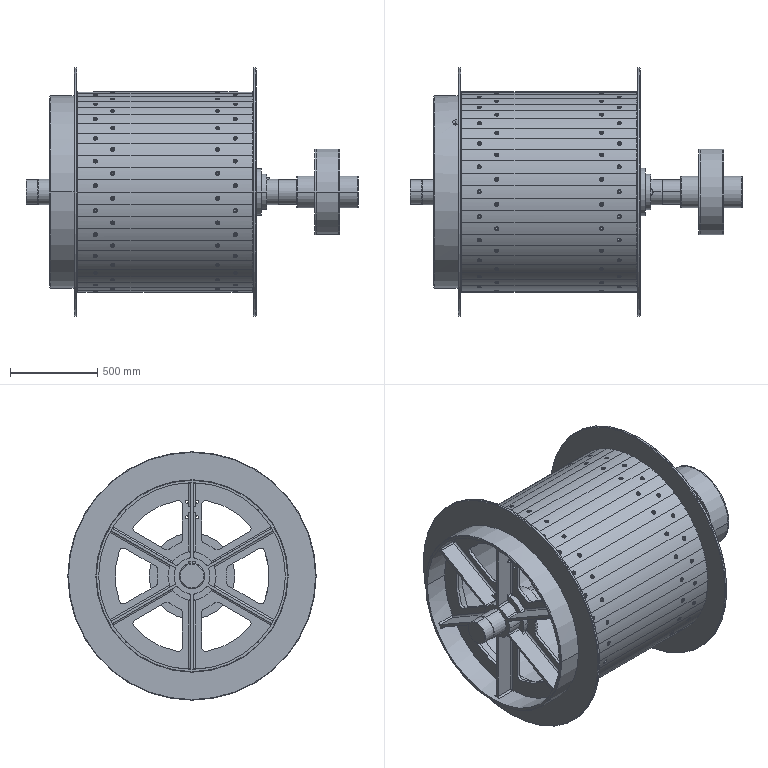Part | SolidWorks | features ReferencePattern 24, LocalCirPattern 1 | 62 solids | 1422 faces | box 1899 x 1420 x 1420 mm | volume 323309066 mm3 | cylinder 894 | plane 419 | cone 71 | torus 38 | commonest cylinder face diameters 13.5 x200 23.78 x200 40 x67 20 x56 50 x56 1046 x52